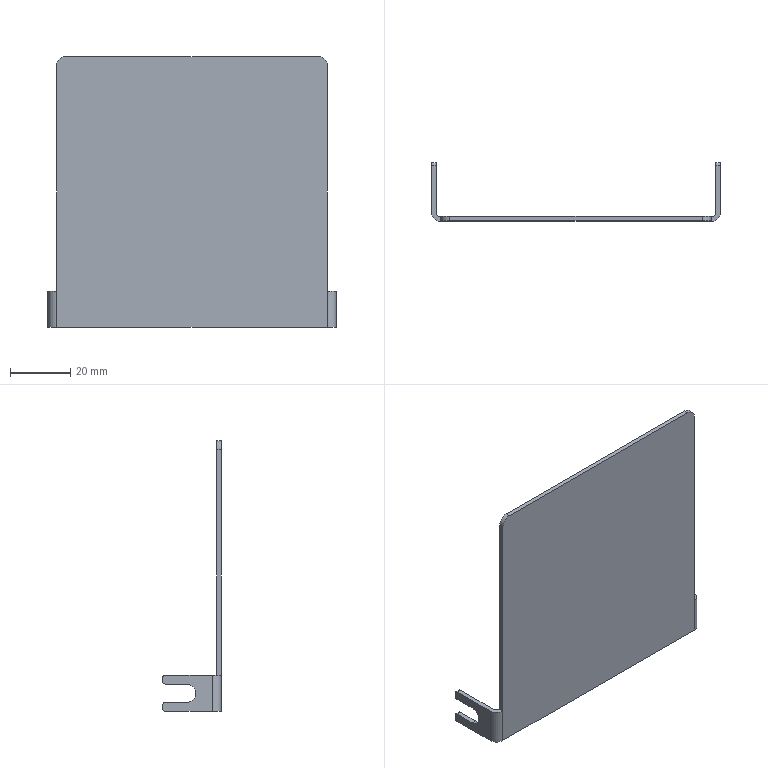Part | NX | features BREP 1 | 1 solid | 36 faces | box 96 x 19.5 x 90 mm | volume 12676 mm3 | plane 20 | cylinder 16 | commonest cylinder face diameters 2 x8 6 x6 3 x2
STEP:
#1=CARTESIAN_POINT('',(45.,0.,0.));
#2=VERTEX_POINT('',#1);
#3=CARTESIAN_POINT('',(-45.,0.,0.));
#4=VERTEX_POINT('',#3);
#5=CARTESIAN_POINT('',(-46.5,0.,0.));
#6=DIRECTION('',(-1.,0.,0.));
#7=VECTOR('',#6,1000.);
#8=LINE('',#5,#7);
#9=EDGE_CURVE('',#2,#4,#8,.T.);
#10=ORIENTED_EDGE('',*,*,#9,.T.);
#11=CARTESIAN_POINT('',(-45.,0.,12.));
#12=VERTEX_POINT('',#11);
#13=CARTESIAN_POINT('',(-45.,0.,90.));
#14=DIRECTION('',(0.,0.,1.));
#15=VECTOR('',#14,1000.);
#16=LINE('',#13,#15);
#17=EDGE_CURVE('',#4,#12,#16,.T.);
#18=ORIENTED_EDGE('',*,*,#17,.T.);
#19=CARTESIAN_POINT('',(-45.,0.,87.));
#20=VERTEX_POINT('',#19);
#21=CARTESIAN_POINT('',(-45.,0.,90.));
#22=DIRECTION('',(0.,0.,1.));
#23=VECTOR('',#22,1000.);
#24=LINE('',#21,#23);
#25=EDGE_CURVE('',#12,#20,#24,.T.);
#26=ORIENTED_EDGE('',*,*,#25,.T.);
#27=CARTESIAN_POINT('',(-42.,0.,90.));
#28=VERTEX_POINT('',#27);
#29=CARTESIAN_POINT('',(-42.,0.,87.));
#30=DIRECTION('',(0.,1.,0.));
#31=DIRECTION('',(1.,0.,0.));
#32=AXIS2_PLACEMENT_3D('',#29,#30,#31);
#33=CIRCLE('',#32,3.);
#34=EDGE_CURVE('',#20,#28,#33,.T.);
#35=ORIENTED_EDGE('',*,*,#34,.T.);
#36=CARTESIAN_POINT('',(42.,0.,90.));
#37=VERTEX_POINT('',#36);
#38=CARTESIAN_POINT('',(-46.5,0.,90.));
#39=DIRECTION('',(1.,0.,0.));
#40=VECTOR('',#39,1000.);
#41=LINE('',#38,#40);
#42=EDGE_CURVE('',#28,#37,#41,.T.);
#43=ORIENTED_EDGE('',*,*,#42,.T.);
#44=CARTESIAN_POINT('',(45.,0.,87.));
#45=VERTEX_POINT('',#44);
#46=CARTESIAN_POINT('',(42.,0.,87.));
#47=DIRECTION('',(0.,1.,0.));
#48=DIRECTION('',(-1.,0.,0.));
#49=AXIS2_PLACEMENT_3D('',#46,#47,#48);
#50=CIRCLE('',#49,3.);
#51=EDGE_CURVE('',#37,#45,#50,.T.);
#52=ORIENTED_EDGE('',*,*,#51,.T.);
#53=CARTESIAN_POINT('',(45.,0.,12.));
#54=VERTEX_POINT('',#53);
#55=CARTESIAN_POINT('',(45.,0.,90.));
#56=DIRECTION('',(0.,0.,-1.));
#57=VECTOR('',#56,1000.);
#58=LINE('',#55,#57);
#59=EDGE_CURVE('',#45,#54,#58,.T.);
#60=ORIENTED_EDGE('',*,*,#59,.T.);
#61=CARTESIAN_POINT('',(45.,0.,90.));
#62=DIRECTION('',(0.,0.,-1.));
#63=VECTOR('',#62,1000.);
#64=LINE('',#61,#63);
#65=EDGE_CURVE('',#54,#2,#64,.T.);
#66=ORIENTED_EDGE('',*,*,#65,.T.);
#67=EDGE_LOOP('',(#10,#18,#26,#35,#43,#52,#60,#66));
#68=FACE_BOUND('',#67,.T.);
#69=CARTESIAN_POINT('',(-46.5,0.,90.));
#70=DIRECTION('',(0.,1.,0.));
#71=DIRECTION('',(1.,0.,0.));
#72=AXIS2_PLACEMENT_3D('',#69,#70,#71);
#73=PLANE('',#72);
#74=ADVANCED_FACE('',(#68),#73,.T.);
#75=CARTESIAN_POINT('',(-46.5,1.5,12.));
#76=VERTEX_POINT('',#75);
#77=CARTESIAN_POINT('',(-45.,1.5,12.));
#78=DIRECTION('',(0.,0.,-1.));
#79=DIRECTION('',(-1.,0.,0.));
#80=AXIS2_PLACEMENT_3D('',#77,#78,#79);
#81=CIRCLE('',#80,1.5);
#82=EDGE_CURVE('',#12,#76,#81,.T.);
#83=ORIENTED_EDGE('',*,*,#82,.F.);
#84=ORIENTED_EDGE('',*,*,#17,.F.);
#85=CARTESIAN_POINT('',(-46.5,1.5,0.));
#86=VERTEX_POINT('',#85);
#87=CARTESIAN_POINT('',(-45.,1.5,0.));
#88=DIRECTION('',(0.,0.,1.));
#89=DIRECTION('',(-1.,0.,0.));
#90=AXIS2_PLACEMENT_3D('',#87,#88,#89);
#91=CIRCLE('',#90,1.5);
#92=EDGE_CURVE('',#86,#4,#91,.T.);
#93=ORIENTED_EDGE('',*,*,#92,.F.);
#94=CARTESIAN_POINT('',(-46.5,1.5,90.));
#95=DIRECTION('',(0.,0.,-1.));
#96=VECTOR('',#95,1000.);
#97=LINE('',#94,#96);
#98=EDGE_CURVE('',#76,#86,#97,.T.);
#99=ORIENTED_EDGE('',*,*,#98,.F.);
#100=EDGE_LOOP('',(#83,#84,#93,#99));
#101=FACE_BOUND('',#100,.T.);
#102=CARTESIAN_POINT('',(-45.,1.5,90.));
#103=DIRECTION('',(0.,0.,-1.));
#104=DIRECTION('',(1.,0.,0.));
#105=AXIS2_PLACEMENT_3D('',#102,#103,#104);
#106=CYLINDRICAL_SURFACE('',#105,1.5);
#107=ADVANCED_FACE('',(#101),#106,.F.);
#108=CARTESIAN_POINT('',(45.,-1.5,0.));
#109=VERTEX_POINT('',#108);
#110=CARTESIAN_POINT('',(-45.,-1.5,0.));
#111=VERTEX_POINT('',#110);
#112=CARTESIAN_POINT('',(48.,-1.5,0.));
#113=DIRECTION('',(-1.,0.,0.));
#114=VECTOR('',#113,1000.);
#115=LINE('',#112,#114);
#116=EDGE_CURVE('',#109,#111,#115,.T.);
#117=ORIENTED_EDGE('',*,*,#116,.T.);
#118=CARTESIAN_POINT('',(-48.,1.5,0.));
#119=VERTEX_POINT('',#118);
#120=CARTESIAN_POINT('',(-45.,1.5,0.));
#121=DIRECTION('',(0.,0.,-1.));
#122=DIRECTION('',(-1.,0.,0.));
#123=AXIS2_PLACEMENT_3D('',#120,#121,#122);
#124=CIRCLE('',#123,3.);
#125=EDGE_CURVE('',#111,#119,#124,.T.);
#126=ORIENTED_EDGE('',*,*,#125,.T.);
#127=CARTESIAN_POINT('',(-48.,17.,0.));
#128=VERTEX_POINT('',#127);
#129=CARTESIAN_POINT('',(-48.,-1.5,0.));
#130=DIRECTION('',(0.,1.,0.));
#131=VECTOR('',#130,1000.);
#132=LINE('',#129,#131);
#133=EDGE_CURVE('',#119,#128,#132,.T.);
#134=ORIENTED_EDGE('',*,*,#133,.T.);
#135=CARTESIAN_POINT('',(-46.5,17.,0.));
#136=VERTEX_POINT('',#135);
#137=CARTESIAN_POINT('',(-45.,17.,0.));
#138=DIRECTION('',(-1.,0.,0.));
#139=VECTOR('',#138,1000.);
#140=LINE('',#137,#139);
#141=EDGE_CURVE('',#136,#128,#140,.T.);
#142=ORIENTED_EDGE('',*,*,#141,.F.);
#143=CARTESIAN_POINT('',(-46.5,18.,0.));
#144=DIRECTION('',(0.,1.,0.));
#145=VECTOR('',#144,1000.);
#146=LINE('',#143,#145);
#147=EDGE_CURVE('',#86,#136,#146,.T.);
#148=ORIENTED_EDGE('',*,*,#147,.F.);
#149=ORIENTED_EDGE('',*,*,#92,.T.);
#150=ORIENTED_EDGE('',*,*,#9,.F.);
#151=CARTESIAN_POINT('',(46.5,1.5,0.));
#152=VERTEX_POINT('',#151);
#153=CARTESIAN_POINT('',(45.,1.5,0.));
#154=DIRECTION('',(0.,0.,1.));
#155=DIRECTION('',(-1.,0.,0.));
#156=AXIS2_PLACEMENT_3D('',#153,#154,#155);
#157=CIRCLE('',#156,1.5);
#158=EDGE_CURVE('',#2,#152,#157,.T.);
#159=ORIENTED_EDGE('',*,*,#158,.T.);
#160=CARTESIAN_POINT('',(46.5,17.,0.));
#161=VERTEX_POINT('',#160);
#162=CARTESIAN_POINT('',(46.5,0.,0.));
#163=DIRECTION('',(0.,-1.,0.));
#164=VECTOR('',#163,1000.);
#165=LINE('',#162,#164);
#166=EDGE_CURVE('',#161,#152,#165,.T.);
#167=ORIENTED_EDGE('',*,*,#166,.F.);
#168=CARTESIAN_POINT('',(48.,17.,0.));
#169=VERTEX_POINT('',#168);
#170=CARTESIAN_POINT('',(45.,17.,0.));
#171=DIRECTION('',(1.,0.,0.));
#172=VECTOR('',#171,1000.);
#173=LINE('',#170,#172);
#174=EDGE_CURVE('',#161,#169,#173,.T.);
#175=ORIENTED_EDGE('',*,*,#174,.T.);
#176=CARTESIAN_POINT('',(48.,1.5,0.));
#177=VERTEX_POINT('',#176);
#178=CARTESIAN_POINT('',(48.,0.,0.));
#179=DIRECTION('',(0.,-1.,0.));
#180=VECTOR('',#179,1000.);
#181=LINE('',#178,#180);
#182=EDGE_CURVE('',#169,#177,#181,.T.);
#183=ORIENTED_EDGE('',*,*,#182,.T.);
#184=CARTESIAN_POINT('',(45.,1.5,0.));
#185=DIRECTION('',(0.,0.,-1.));
#186=DIRECTION('',(-1.,0.,0.));
#187=AXIS2_PLACEMENT_3D('',#184,#185,#186);
#188=CIRCLE('',#187,3.);
#189=EDGE_CURVE('',#177,#109,#188,.T.);
#190=ORIENTED_EDGE('',*,*,#189,.T.);
#191=EDGE_LOOP('',(#117,#126,#134,#142,#148,#149,#150,#159,#167,#175,#183,#190));
#192=FACE_BOUND('',#191,.T.);
#193=CARTESIAN_POINT('',(48.,1.5,0.));
#194=DIRECTION('',(0.,0.,-1.));
#195=DIRECTION('',(1.,0.,0.));
#196=AXIS2_PLACEMENT_3D('',#193,#194,#195);
#197=PLANE('',#196);
#198=ADVANCED_FACE('',(#192),#197,.T.);
#199=CARTESIAN_POINT('',(46.5,1.5,12.));
#200=VERTEX_POINT('',#199);
#201=CARTESIAN_POINT('',(46.5,1.5,90.));
#202=DIRECTION('',(0.,0.,1.));
#203=VECTOR('',#202,1000.);
#204=LINE('',#201,#203);
#205=EDGE_CURVE('',#152,#200,#204,.T.);
#206=ORIENTED_EDGE('',*,*,#205,.F.);
#207=ORIENTED_EDGE('',*,*,#158,.F.);
#208=ORIENTED_EDGE('',*,*,#65,.F.);
#209=CARTESIAN_POINT('',(45.,1.5,12.));
#210=DIRECTION('',(0.,0.,-1.));
#211=DIRECTION('',(-1.,0.,0.));
#212=AXIS2_PLACEMENT_3D('',#209,#210,#211);
#213=CIRCLE('',#212,1.5);
#214=EDGE_CURVE('',#200,#54,#213,.T.);
#215=ORIENTED_EDGE('',*,*,#214,.F.);
#216=EDGE_LOOP('',(#206,#207,#208,#215));
#217=FACE_BOUND('',#216,.T.);
#218=CARTESIAN_POINT('',(45.,1.5,90.));
#219=DIRECTION('',(0.,0.,-1.));
#220=DIRECTION('',(1.,0.,0.));
#221=AXIS2_PLACEMENT_3D('',#218,#219,#220);
#222=CYLINDRICAL_SURFACE('',#221,1.5);
#223=ADVANCED_FACE('',(#217),#222,.F.);
#224=CARTESIAN_POINT('',(45.,-1.5,87.));
#225=VERTEX_POINT('',#224);
#226=CARTESIAN_POINT('',(45.,-1.5,12.));
#227=VERTEX_POINT('',#226);
#228=CARTESIAN_POINT('',(45.,-1.5,0.));
#229=DIRECTION('',(0.,0.,-1.));
#230=VECTOR('',#229,1000.);
#231=LINE('',#228,#230);
#232=EDGE_CURVE('',#225,#227,#231,.T.);
#233=ORIENTED_EDGE('',*,*,#232,.T.);
#234=CARTESIAN_POINT('',(45.,0.,12.));
#235=DIRECTION('',(0.,1.,0.));
#236=VECTOR('',#235,1000.);
#237=LINE('',#234,#236);
#238=EDGE_CURVE('',#227,#54,#237,.T.);
#239=ORIENTED_EDGE('',*,*,#238,.T.);
#240=ORIENTED_EDGE('',*,*,#59,.F.);
#241=CARTESIAN_POINT('',(45.,0.,87.));
#242=DIRECTION('',(0.,-1.,0.));
#243=VECTOR('',#242,1000.);
#244=LINE('',#241,#243);
#245=EDGE_CURVE('',#45,#225,#244,.T.);
#246=ORIENTED_EDGE('',*,*,#245,.T.);
#247=EDGE_LOOP('',(#233,#239,#240,#246));
#248=FACE_BOUND('',#247,.T.);
#249=CARTESIAN_POINT('',(45.,0.,0.));
#250=DIRECTION('',(1.,0.,0.));
#251=DIRECTION('',(0.,-1.,0.));
#252=AXIS2_PLACEMENT_3D('',#249,#250,#251);
#253=PLANE('',#252);
#254=ADVANCED_FACE('',(#248),#253,.T.);
#255=ORIENTED_EDGE('',*,*,#51,.F.);
#256=CARTESIAN_POINT('',(42.,-1.5,90.));
#257=VERTEX_POINT('',#256);
#258=CARTESIAN_POINT('',(42.,1.5,90.));
#259=DIRECTION('',(0.,-1.,0.));
#260=VECTOR('',#259,1000.);
#261=LINE('',#258,#260);
#262=EDGE_CURVE('',#37,#257,#261,.T.);
#263=ORIENTED_EDGE('',*,*,#262,.T.);
#264=CARTESIAN_POINT('',(42.,-1.5,87.));
#265=DIRECTION('',(0.,1.,0.));
#266=DIRECTION('',(-1.,0.,0.));
#267=AXIS2_PLACEMENT_3D('',#264,#265,#266);
#268=CIRCLE('',#267,3.);
#269=EDGE_CURVE('',#257,#225,#268,.T.);
#270=ORIENTED_EDGE('',*,*,#269,.T.);
#271=ORIENTED_EDGE('',*,*,#245,.F.);
#272=EDGE_LOOP('',(#255,#263,#270,#271));
#273=FACE_BOUND('',#272,.T.);
#274=CARTESIAN_POINT('',(42.,1.5,87.));
#275=DIRECTION('',(0.,1.,0.));
#276=DIRECTION('',(1.,0.,0.));
#277=AXIS2_PLACEMENT_3D('',#274,#275,#276);
#278=CYLINDRICAL_SURFACE('',#277,3.);
#279=ADVANCED_FACE('',(#273),#278,.T.);
#280=CARTESIAN_POINT('',(-42.,-1.5,90.));
#281=VERTEX_POINT('',#280);
#282=CARTESIAN_POINT('',(-48.,-1.5,90.));
#283=DIRECTION('',(1.,0.,0.));
#284=VECTOR('',#283,1000.);
#285=LINE('',#282,#284);
#286=EDGE_CURVE('',#281,#257,#285,.T.);
#287=ORIENTED_EDGE('',*,*,#286,.T.);
#288=ORIENTED_EDGE('',*,*,#262,.F.);
#289=ORIENTED_EDGE('',*,*,#42,.F.);
#290=CARTESIAN_POINT('',(-42.,1.5,90.));
#291=DIRECTION('',(0.,-1.,0.));
#292=VECTOR('',#291,1000.);
#293=LINE('',#290,#292);
#294=EDGE_CURVE('',#28,#281,#293,.T.);
#295=ORIENTED_EDGE('',*,*,#294,.T.);
#296=EDGE_LOOP('',(#287,#288,#289,#295));
#297=FACE_BOUND('',#296,.T.);
#298=CARTESIAN_POINT('',(-48.,1.5,90.));
#299=DIRECTION('',(0.,0.,1.));
#300=DIRECTION('',(-1.,0.,0.));
#301=AXIS2_PLACEMENT_3D('',#298,#299,#300);
#302=PLANE('',#301);
#303=ADVANCED_FACE('',(#297),#302,.T.);
#304=CARTESIAN_POINT('',(-45.,-1.5,87.));
#305=VERTEX_POINT('',#304);
#306=CARTESIAN_POINT('',(-42.,-1.5,87.));
#307=DIRECTION('',(0.,1.,0.));
#308=DIRECTION('',(1.,0.,0.));
#309=AXIS2_PLACEMENT_3D('',#306,#307,#308);
#310=CIRCLE('',#309,3.);
#311=EDGE_CURVE('',#305,#281,#310,.T.);
#312=ORIENTED_EDGE('',*,*,#311,.T.);
#313=ORIENTED_EDGE('',*,*,#294,.F.);
#314=ORIENTED_EDGE('',*,*,#34,.F.);
#315=CARTESIAN_POINT('',(-45.,1.5,87.));
#316=DIRECTION('',(0.,-1.,0.));
#317=VECTOR('',#316,1000.);
#318=LINE('',#315,#317);
#319=EDGE_CURVE('',#20,#305,#318,.T.);
#320=ORIENTED_EDGE('',*,*,#319,.T.);
#321=EDGE_LOOP('',(#312,#313,#314,#320));
#322=FACE_BOUND('',#321,.T.);
#323=CARTESIAN_POINT('',(-42.,1.5,87.));
#324=DIRECTION('',(0.,-1.,0.));
#325=DIRECTION('',(-1.,0.,0.));
#326=AXIS2_PLACEMENT_3D('',#323,#324,#325);
#327=CYLINDRICAL_SURFACE('',#326,3.);
#328=ADVANCED_FACE('',(#322),#327,.T.);
#329=ORIENTED_EDGE('',*,*,#25,.F.);
#330=CARTESIAN_POINT('',(-45.,-1.5,12.));
#331=VERTEX_POINT('',#330);
#332=CARTESIAN_POINT('',(-45.,0.,12.));
#333=DIRECTION('',(0.,-1.,0.));
#334=VECTOR('',#333,1000.);
#335=LINE('',#332,#334);
#336=EDGE_CURVE('',#12,#331,#335,.T.);
#337=ORIENTED_EDGE('',*,*,#336,.T.);
#338=CARTESIAN_POINT('',(-45.,-1.5,0.));
#339=DIRECTION('',(0.,0.,1.));
#340=VECTOR('',#339,1000.);
#341=LINE('',#338,#340);
#342=EDGE_CURVE('',#331,#305,#341,.T.);
#343=ORIENTED_EDGE('',*,*,#342,.T.);
#344=ORIENTED_EDGE('',*,*,#319,.F.);
#345=EDGE_LOOP('',(#329,#337,#343,#344));
#346=FACE_BOUND('',#345,.T.);
#347=CARTESIAN_POINT('',(-45.,0.,0.));
#348=DIRECTION('',(-1.,0.,0.));
#349=DIRECTION('',(0.,1.,0.));
#350=AXIS2_PLACEMENT_3D('',#347,#348,#349);
#351=PLANE('',#350);
#352=ADVANCED_FACE('',(#346),#351,.T.);
#353=CARTESIAN_POINT('',(-46.5,17.,12.));
#354=VERTEX_POINT('',#353);
#355=CARTESIAN_POINT('',(-46.5,18.,12.));
#356=DIRECTION('',(0.,-1.,0.));
#357=VECTOR('',#356,1000.);
#358=LINE('',#355,#357);
#359=EDGE_CURVE('',#354,#76,#358,.T.);
#360=ORIENTED_EDGE('',*,*,#359,.T.);
#361=ORIENTED_EDGE('',*,*,#98,.T.);
#362=ORIENTED_EDGE('',*,*,#147,.T.);
#363=CARTESIAN_POINT('',(-46.5,18.,1.));
#364=VERTEX_POINT('',#363);
#365=CARTESIAN_POINT('',(-46.5,17.,1.));
#366=DIRECTION('',(1.,0.,0.));
#367=DIRECTION('',(0.,0.,-1.));
#368=AXIS2_PLACEMENT_3D('',#365,#366,#367);
#369=CIRCLE('',#368,1.);
#370=EDGE_CURVE('',#136,#364,#369,.T.);
#371=ORIENTED_EDGE('',*,*,#370,.T.);
#372=CARTESIAN_POINT('',(-46.5,18.,2.));
#373=VERTEX_POINT('',#372);
#374=CARTESIAN_POINT('',(-46.5,18.,90.));
#375=DIRECTION('',(0.,0.,1.));
#376=VECTOR('',#375,1000.);
#377=LINE('',#374,#376);
#378=EDGE_CURVE('',#364,#373,#377,.T.);
#379=ORIENTED_EDGE('',*,*,#378,.T.);
#380=CARTESIAN_POINT('',(-46.5,17.,3.));
#381=VERTEX_POINT('',#380);
#382=CARTESIAN_POINT('',(-46.5,17.,2.));
#383=DIRECTION('',(1.,0.,0.));
#384=DIRECTION('',(0.,0.,1.));
#385=AXIS2_PLACEMENT_3D('',#382,#383,#384);
#386=CIRCLE('',#385,1.);
#387=EDGE_CURVE('',#373,#381,#386,.T.);
#388=ORIENTED_EDGE('',*,*,#387,.T.);
#389=CARTESIAN_POINT('',(-46.5,10.,3.));
#390=VERTEX_POINT('',#389);
#391=CARTESIAN_POINT('',(-46.5,18.,3.));
#392=DIRECTION('',(0.,-1.,0.));
#393=VECTOR('',#392,1000.);
#394=LINE('',#391,#393);
#395=EDGE_CURVE('',#381,#390,#394,.T.);
#396=ORIENTED_EDGE('',*,*,#395,.T.);
#397=CARTESIAN_POINT('',(-46.5,10.,9.));
#398=VERTEX_POINT('',#397);
#399=CARTESIAN_POINT('',(-46.5,10.,6.));
#400=DIRECTION('',(-1.,0.,0.));
#401=DIRECTION('',(0.,1.,0.));
#402=AXIS2_PLACEMENT_3D('',#399,#400,#401);
#403=CIRCLE('',#402,3.);
#404=EDGE_CURVE('',#390,#398,#403,.T.);
#405=ORIENTED_EDGE('',*,*,#404,.T.);
#406=CARTESIAN_POINT('',(-46.5,17.,9.));
#407=VERTEX_POINT('',#406);
#408=CARTESIAN_POINT('',(-46.5,18.,9.));
#409=DIRECTION('',(0.,1.,0.));
#410=VECTOR('',#409,1000.);
#411=LINE('',#408,#410);
#412=EDGE_CURVE('',#398,#407,#411,.T.);
#413=ORIENTED_EDGE('',*,*,#412,.T.);
#414=CARTESIAN_POINT('',(-46.5,18.,10.));
#415=VERTEX_POINT('',#414);
#416=CARTESIAN_POINT('',(-46.5,17.,10.));
#417=DIRECTION('',(1.,0.,0.));
#418=DIRECTION('',(0.,0.,1.));
#419=AXIS2_PLACEMENT_3D('',#416,#417,#418);
#420=CIRCLE('',#419,1.);
#421=EDGE_CURVE('',#407,#415,#420,.T.);
#422=ORIENTED_EDGE('',*,*,#421,.T.);
#423=CARTESIAN_POINT('',(-46.5,18.,11.));
#424=VERTEX_POINT('',#423);
#425=CARTESIAN_POINT('',(-46.5,18.,90.));
#426=DIRECTION('',(0.,0.,1.));
#427=VECTOR('',#426,1000.);
#428=LINE('',#425,#427);
#429=EDGE_CURVE('',#415,#424,#428,.T.);
#430=ORIENTED_EDGE('',*,*,#429,.T.);
#431=CARTESIAN_POINT('',(-46.5,17.,11.));
#432=DIRECTION('',(1.,0.,0.));
#433=DIRECTION('',(0.,0.,1.));
#434=AXIS2_PLACEMENT_3D('',#431,#432,#433);
#435=CIRCLE('',#434,1.);
#436=EDGE_CURVE('',#424,#354,#435,.T.);
#437=ORIENTED_EDGE('',*,*,#436,.T.);
#438=EDGE_LOOP('',(#360,#361,#362,#371,#379,#388,#396,#405,#413,#422,#430,#437));
#439=FACE_BOUND('',#438,.T.);
#440=CARTESIAN_POINT('',(-46.5,18.,90.));
#441=DIRECTION('',(1.,0.,0.));
#442=DIRECTION('',(0.,-1.,0.));
#443=AXIS2_PLACEMENT_3D('',#440,#441,#442);
#444=PLANE('',#443);
#445=ADVANCED_FACE('',(#439),#444,.T.);
#446=ORIENTED_EDGE('',*,*,#336,.F.);
#447=ORIENTED_EDGE('',*,*,#82,.T.);
#448=ORIENTED_EDGE('',*,*,#359,.F.);
#449=CARTESIAN_POINT('',(-48.,17.,12.));
#450=VERTEX_POINT('',#449);
#451=CARTESIAN_POINT('',(-45.,17.,12.));
#452=DIRECTION('',(-1.,0.,0.));
#453=VECTOR('',#452,1000.);
#454=LINE('',#451,#453);
#455=EDGE_CURVE('',#354,#450,#454,.T.);
#456=ORIENTED_EDGE('',*,*,#455,.T.);
#457=CARTESIAN_POINT('',(-48.,1.5,12.));
#458=VERTEX_POINT('',#457);
#459=CARTESIAN_POINT('',(-48.,-1.5,12.));
#460=DIRECTION('',(0.,-1.,0.));
#461=VECTOR('',#460,1000.);
#462=LINE('',#459,#461);
#463=EDGE_CURVE('',#450,#458,#462,.T.);
#464=ORIENTED_EDGE('',*,*,#463,.T.);
#465=CARTESIAN_POINT('',(-45.,1.5,12.));
#466=DIRECTION('',(0.,0.,1.));
#467=DIRECTION('',(-1.,0.,0.));
#468=AXIS2_PLACEMENT_3D('',#465,#466,#467);
#469=CIRCLE('',#468,3.);
#470=EDGE_CURVE('',#458,#331,#469,.T.);
#471=ORIENTED_EDGE('',*,*,#470,.T.);
#472=EDGE_LOOP('',(#446,#447,#448,#456,#464,#471));
#473=FACE_BOUND('',#472,.T.);
#474=CARTESIAN_POINT('',(-45.,-1.5,12.));
#475=DIRECTION('',(0.,0.,1.));
#476=DIRECTION('',(-1.,0.,0.));
#477=AXIS2_PLACEMENT_3D('',#474,#475,#476);
#478=PLANE('',#477);
#479=ADVANCED_FACE('',(#473),#478,.T.);
#480=ORIENTED_EDGE('',*,*,#311,.F.);
#481=ORIENTED_EDGE('',*,*,#342,.F.);
#482=CARTESIAN_POINT('',(-45.,-1.5,90.));
#483=DIRECTION('',(0.,0.,1.));
#484=VECTOR('',#483,1000.);
#485=LINE('',#482,#484);
#486=EDGE_CURVE('',#111,#331,#485,.T.);
#487=ORIENTED_EDGE('',*,*,#486,.F.);
#488=ORIENTED_EDGE('',*,*,#116,.F.);
#489=CARTESIAN_POINT('',(45.,-1.5,90.));
#490=DIRECTION('',(0.,0.,-1.));
#491=VECTOR('',#490,1000.);
#492=LINE('',#489,#491);
#493=EDGE_CURVE('',#227,#109,#492,.T.);
#494=ORIENTED_EDGE('',*,*,#493,.F.);
#495=ORIENTED_EDGE('',*,*,#232,.F.);
#496=ORIENTED_EDGE('',*,*,#269,.F.);
#497=ORIENTED_EDGE('',*,*,#286,.F.);
#498=EDGE_LOOP('',(#480,#481,#487,#488,#494,#495,#496,#497));
#499=FACE_BOUND('',#498,.T.);
#500=CARTESIAN_POINT('',(-46.5,-1.5,90.));
#501=DIRECTION('',(0.,1.,0.));
#502=DIRECTION('',(1.,0.,0.));
#503=AXIS2_PLACEMENT_3D('',#500,#501,#502);
#504=PLANE('',#503);
#505=ADVANCED_FACE('',(#499),#504,.F.);
#506=CARTESIAN_POINT('',(46.5,17.,12.));
#507=VERTEX_POINT('',#506);
#508=CARTESIAN_POINT('',(48.,17.,12.));
#509=VERTEX_POINT('',#508);
#510=CARTESIAN_POINT('',(45.,17.,12.));
#511=DIRECTION('',(1.,0.,0.));
#512=VECTOR('',#511,1000.);
#513=LINE('',#510,#512);
#514=EDGE_CURVE('',#507,#509,#513,.T.);
#515=ORIENTED_EDGE('',*,*,#514,.F.);
#516=CARTESIAN_POINT('',(46.5,-1.5,12.));
#517=DIRECTION('',(0.,1.,0.));
#518=VECTOR('',#517,1000.);
#519=LINE('',#516,#518);
#520=EDGE_CURVE('',#200,#507,#519,.T.);
#521=ORIENTED_EDGE('',*,*,#520,.F.);
#522=ORIENTED_EDGE('',*,*,#214,.T.);
#523=ORIENTED_EDGE('',*,*,#238,.F.);
#524=CARTESIAN_POINT('',(48.,1.5,12.));
#525=VERTEX_POINT('',#524);
#526=CARTESIAN_POINT('',(45.,1.5,12.));
#527=DIRECTION('',(0.,0.,-1.));
#528=DIRECTION('',(-1.,0.,0.));
#529=AXIS2_PLACEMENT_3D('',#526,#527,#528);
#530=CIRCLE('',#529,3.);
#531=EDGE_CURVE('',#525,#227,#530,.T.);
#532=ORIENTED_EDGE('',*,*,#531,.F.);
#533=CARTESIAN_POINT('',(48.,-1.5,12.));
#534=DIRECTION('',(0.,-1.,0.));
#535=VECTOR('',#534,1000.);
#536=LINE('',#533,#535);
#537=EDGE_CURVE('',#509,#525,#536,.T.);
#538=ORIENTED_EDGE('',*,*,#537,.F.);
#539=EDGE_LOOP('',(#515,#521,#522,#523,#532,#538));
#540=FACE_BOUND('',#539,.T.);
#541=CARTESIAN_POINT('',(45.,-1.5,12.));
#542=DIRECTION('',(0.,0.,-1.));
#543=DIRECTION('',(1.,0.,0.));
#544=AXIS2_PLACEMENT_3D('',#541,#542,#543);
#545=PLANE('',#544);
#546=ADVANCED_FACE('',(#540),#545,.F.);
#547=ORIENTED_EDGE('',*,*,#166,.T.);
#548=ORIENTED_EDGE('',*,*,#205,.T.);
#549=ORIENTED_EDGE('',*,*,#520,.T.);
#550=CARTESIAN_POINT('',(46.5,18.,11.));
#551=VERTEX_POINT('',#550);
#552=CARTESIAN_POINT('',(46.5,17.,11.));
#553=DIRECTION('',(-1.,0.,0.));
#554=DIRECTION('',(0.,0.,1.));
#555=AXIS2_PLACEMENT_3D('',#552,#553,#554);
#556=CIRCLE('',#555,1.);
#557=EDGE_CURVE('',#507,#551,#556,.T.);
#558=ORIENTED_EDGE('',*,*,#557,.T.);
#559=CARTESIAN_POINT('',(46.5,18.,10.));
#560=VERTEX_POINT('',#559);
#561=CARTESIAN_POINT('',(46.5,18.,90.));
#562=DIRECTION('',(0.,0.,-1.));
#563=VECTOR('',#562,1000.);
#564=LINE('',#561,#563);
#565=EDGE_CURVE('',#551,#560,#564,.T.);
#566=ORIENTED_EDGE('',*,*,#565,.T.);
#567=CARTESIAN_POINT('',(46.5,17.,9.));
#568=VERTEX_POINT('',#567);
#569=CARTESIAN_POINT('',(46.5,17.,10.));
#570=DIRECTION('',(-1.,0.,0.));
#571=DIRECTION('',(0.,0.,1.));
#572=AXIS2_PLACEMENT_3D('',#569,#570,#571);
#573=CIRCLE('',#572,1.);
#574=EDGE_CURVE('',#560,#568,#573,.T.);
#575=ORIENTED_EDGE('',*,*,#574,.T.);
#576=CARTESIAN_POINT('',(46.5,10.,9.));
#577=VERTEX_POINT('',#576);
#578=CARTESIAN_POINT('',(46.5,0.,9.));
#579=DIRECTION('',(0.,-1.,0.));
#580=VECTOR('',#579,1000.);
#581=LINE('',#578,#580);
#582=EDGE_CURVE('',#568,#577,#581,.T.);
#583=ORIENTED_EDGE('',*,*,#582,.T.);
#584=CARTESIAN_POINT('',(46.5,10.,3.));
#585=VERTEX_POINT('',#584);
#586=CARTESIAN_POINT('',(46.5,10.,6.));
#587=DIRECTION('',(1.,0.,0.));
#588=DIRECTION('',(0.,1.,0.));
#589=AXIS2_PLACEMENT_3D('',#586,#587,#588);
#590=CIRCLE('',#589,3.);
#591=EDGE_CURVE('',#577,#585,#590,.T.);
#592=ORIENTED_EDGE('',*,*,#591,.T.);
#593=CARTESIAN_POINT('',(46.5,17.,3.));
#594=VERTEX_POINT('',#593);
#595=CARTESIAN_POINT('',(46.5,0.,3.));
#596=DIRECTION('',(0.,1.,0.));
#597=VECTOR('',#596,1000.);
#598=LINE('',#595,#597);
#599=EDGE_CURVE('',#585,#594,#598,.T.);
#600=ORIENTED_EDGE('',*,*,#599,.T.);
#601=CARTESIAN_POINT('',(46.5,18.,2.));
#602=VERTEX_POINT('',#601);
#603=CARTESIAN_POINT('',(46.5,17.,2.));
#604=DIRECTION('',(-1.,0.,0.));
#605=DIRECTION('',(0.,0.,1.));
#606=AXIS2_PLACEMENT_3D('',#603,#604,#605);
#607=CIRCLE('',#606,1.);
#608=EDGE_CURVE('',#594,#602,#607,.T.);
#609=ORIENTED_EDGE('',*,*,#608,.T.);
#610=CARTESIAN_POINT('',(46.5,18.,1.));
#611=VERTEX_POINT('',#610);
#612=CARTESIAN_POINT('',(46.5,18.,90.));
#613=DIRECTION('',(0.,0.,-1.));
#614=VECTOR('',#613,1000.);
#615=LINE('',#612,#614);
#616=EDGE_CURVE('',#602,#611,#615,.T.);
#617=ORIENTED_EDGE('',*,*,#616,.T.);
#618=CARTESIAN_POINT('',(46.5,17.,1.));
#619=DIRECTION('',(-1.,0.,0.));
#620=DIRECTION('',(0.,0.,-1.));
#621=AXIS2_PLACEMENT_3D('',#618,#619,#620);
#622=CIRCLE('',#621,1.);
#623=EDGE_CURVE('',#611,#161,#622,.T.);
#624=ORIENTED_EDGE('',*,*,#623,.T.);
#625=EDGE_LOOP('',(#547,#548,#549,#558,#566,#575,#583,#592,#600,#609,#617,#624));
#626=FACE_BOUND('',#625,.T.);
#627=CARTESIAN_POINT('',(46.5,0.,90.));
#628=DIRECTION('',(-1.,0.,0.));
#629=DIRECTION('',(0.,1.,0.));
#630=AXIS2_PLACEMENT_3D('',#627,#628,#629);
#631=PLANE('',#630);
#632=ADVANCED_FACE('',(#626),#631,.T.);
#633=CARTESIAN_POINT('',(-48.,18.,11.));
#634=VERTEX_POINT('',#633);
#635=CARTESIAN_POINT('',(-48.,17.,11.));
#636=DIRECTION('',(1.,0.,0.));
#637=DIRECTION('',(0.,0.,1.));
#638=AXIS2_PLACEMENT_3D('',#635,#636,#637);
#639=CIRCLE('',#638,1.);
#640=EDGE_CURVE('',#634,#450,#639,.T.);
#641=ORIENTED_EDGE('',*,*,#640,.T.);
#642=ORIENTED_EDGE('',*,*,#455,.F.);
#643=ORIENTED_EDGE('',*,*,#436,.F.);
#644=CARTESIAN_POINT('',(-45.,18.,11.));
#645=DIRECTION('',(-1.,0.,0.));
#646=VECTOR('',#645,1000.);
#647=LINE('',#644,#646);
#648=EDGE_CURVE('',#424,#634,#647,.T.);
#649=ORIENTED_EDGE('',*,*,#648,.T.);
#650=EDGE_LOOP('',(#641,#642,#643,#649));
#651=FACE_BOUND('',#650,.T.);
#652=CARTESIAN_POINT('',(-45.,17.,11.));
#653=DIRECTION('',(-1.,0.,0.));
#654=DIRECTION('',(0.,0.,-1.));
#655=AXIS2_PLACEMENT_3D('',#652,#653,#654);
#656=CYLINDRICAL_SURFACE('',#655,1.);
#657=ADVANCED_FACE('',(#651),#656,.T.);
#658=ORIENTED_EDGE('',*,*,#429,.F.);
#659=CARTESIAN_POINT('',(-48.,18.,10.));
#660=VERTEX_POINT('',#659);
#661=CARTESIAN_POINT('',(-48.,18.,10.));
#662=DIRECTION('',(-1.,0.,0.));
#663=VECTOR('',#662,1000.);
#664=LINE('',#661,#663);
#665=EDGE_CURVE('',#415,#660,#664,.T.);
#666=ORIENTED_EDGE('',*,*,#665,.T.);
#667=CARTESIAN_POINT('',(-48.,18.,90.));
#668=DIRECTION('',(0.,0.,1.));
#669=VECTOR('',#668,1000.);
#670=LINE('',#667,#669);
#671=EDGE_CURVE('',#660,#634,#670,.T.);
#672=ORIENTED_EDGE('',*,*,#671,.T.);
#673=ORIENTED_EDGE('',*,*,#648,.F.);
#674=EDGE_LOOP('',(#658,#666,#672,#673));
#675=FACE_BOUND('',#674,.T.);
#676=CARTESIAN_POINT('',(-48.,18.,90.));
#677=DIRECTION('',(0.,1.,0.));
#678=DIRECTION('',(0.,0.,-1.));
#679=AXIS2_PLACEMENT_3D('',#676,#677,#678);
#680=PLANE('',#679);
#681=ADVANCED_FACE('',(#675),#680,.T.);
#682=ORIENTED_EDGE('',*,*,#421,.F.);
#683=CARTESIAN_POINT('',(-48.,17.,9.));
#684=VERTEX_POINT('',#683);
#685=CARTESIAN_POINT('',(-48.,17.,9.));
#686=DIRECTION('',(-1.,0.,0.));
#687=VECTOR('',#686,1000.);
#688=LINE('',#685,#687);
#689=EDGE_CURVE('',#407,#684,#688,.T.);
#690=ORIENTED_EDGE('',*,*,#689,.T.);
#691=CARTESIAN_POINT('',(-48.,17.,10.));
#692=DIRECTION('',(1.,0.,0.));
#693=DIRECTION('',(0.,0.,1.));
#694=AXIS2_PLACEMENT_3D('',#691,#692,#693);
#695=CIRCLE('',#694,1.);
#696=EDGE_CURVE('',#684,#660,#695,.T.);
#697=ORIENTED_EDGE('',*,*,#696,.T.);
#698=ORIENTED_EDGE('',*,*,#665,.F.);
#699=EDGE_LOOP('',(#682,#690,#697,#698));
#700=FACE_BOUND('',#699,.T.);
#701=CARTESIAN_POINT('',(-48.,17.,10.));
#702=DIRECTION('',(-1.,0.,0.));
#703=DIRECTION('',(0.,0.,-1.));
#704=AXIS2_PLACEMENT_3D('',#701,#702,#703);
#705=CYLINDRICAL_SURFACE('',#704,1.);
#706=ADVANCED_FACE('',(#700),#705,.T.);
#707=ORIENTED_EDGE('',*,*,#689,.F.);
#708=ORIENTED_EDGE('',*,*,#412,.F.);
#709=CARTESIAN_POINT('',(-48.,10.,9.));
#710=VERTEX_POINT('',#709);
#711=CARTESIAN_POINT('',(-48.,10.,9.));
#712=DIRECTION('',(1.,0.,0.));
#713=VECTOR('',#712,1000.);
#714=LINE('',#711,#713);
#715=EDGE_CURVE('',#710,#398,#714,.T.);
#716=ORIENTED_EDGE('',*,*,#715,.F.);
#717=CARTESIAN_POINT('',(-48.,18.,9.));
#718=DIRECTION('',(0.,-1.,0.));
#719=VECTOR('',#718,1000.);
#720=LINE('',#717,#719);
#721=EDGE_CURVE('',#684,#710,#720,.T.);
#722=ORIENTED_EDGE('',*,*,#721,.F.);
#723=EDGE_LOOP('',(#707,#708,#716,#722));
#724=FACE_BOUND('',#723,.T.);
#725=CARTESIAN_POINT('',(-48.,18.,9.));
#726=DIRECTION('',(0.,0.,1.));
#727=DIRECTION('',(-1.,0.,0.));
#728=AXIS2_PLACEMENT_3D('',#725,#726,#727);
#729=PLANE('',#728);
#730=ADVANCED_FACE('',(#724),#729,.F.);
#731=CARTESIAN_POINT('',(-48.,10.,3.));
#732=VERTEX_POINT('',#731);
#733=CARTESIAN_POINT('',(-48.,10.,3.));
#734=DIRECTION('',(1.,0.,0.));
#735=VECTOR('',#734,1000.);
#736=LINE('',#733,#735);
#737=EDGE_CURVE('',#732,#390,#736,.T.);
#738=ORIENTED_EDGE('',*,*,#737,.F.);
#739=CARTESIAN_POINT('',(-48.,10.,6.));
#740=DIRECTION('',(1.,0.,0.));
#741=DIRECTION('',(0.,1.,0.));
#742=AXIS2_PLACEMENT_3D('',#739,#740,#741);
#743=CIRCLE('',#742,3.);
#744=EDGE_CURVE('',#710,#732,#743,.T.);
#745=ORIENTED_EDGE('',*,*,#744,.F.);
#746=ORIENTED_EDGE('',*,*,#715,.T.);
#747=ORIENTED_EDGE('',*,*,#404,.F.);
#748=EDGE_LOOP('',(#738,#745,#746,#747));
#749=FACE_BOUND('',#748,.T.);
#750=CARTESIAN_POINT('',(-48.,10.,6.));
#751=DIRECTION('',(1.,0.,0.));
#752=DIRECTION('',(0.,-1.,0.));
#753=AXIS2_PLACEMENT_3D('',#750,#751,#752);
#754=CYLINDRICAL_SURFACE('',#753,3.);
#755=ADVANCED_FACE('',(#749),#754,.F.);
#756=CARTESIAN_POINT('',(-48.,17.,3.));
#757=VERTEX_POINT('',#756);
#758=CARTESIAN_POINT('',(-48.,17.,3.));
#759=DIRECTION('',(1.,0.,0.));
#760=VECTOR('',#759,1000.);
#761=LINE('',#758,#760);
#762=EDGE_CURVE('',#757,#381,#761,.T.);
#763=ORIENTED_EDGE('',*,*,#762,.F.);
#764=CARTESIAN_POINT('',(-48.,18.,3.));
#765=DIRECTION('',(0.,1.,0.));
#766=VECTOR('',#765,1000.);
#767=LINE('',#764,#766);
#768=EDGE_CURVE('',#732,#757,#767,.T.);
#769=ORIENTED_EDGE('',*,*,#768,.F.);
#770=ORIENTED_EDGE('',*,*,#737,.T.);
#771=ORIENTED_EDGE('',*,*,#395,.F.);
#772=EDGE_LOOP('',(#763,#769,#770,#771));
#773=FACE_BOUND('',#772,.T.);
#774=CARTESIAN_POINT('',(-48.,18.,3.));
#775=DIRECTION('',(0.,0.,-1.));
#776=DIRECTION('',(0.,-1.,0.));
#777=AXIS2_PLACEMENT_3D('',#774,#775,#776);
#778=PLANE('',#777);
#779=ADVANCED_FACE('',(#773),#778,.F.);
#780=ORIENTED_EDGE('',*,*,#387,.F.);
#781=CARTESIAN_POINT('',(-48.,18.,2.));
#782=VERTEX_POINT('',#781);
#783=CARTESIAN_POINT('',(-48.,18.,2.));
#784=DIRECTION('',(-1.,0.,0.));
#785=VECTOR('',#784,1000.);
#786=LINE('',#783,#785);
#787=EDGE_CURVE('',#373,#782,#786,.T.);
#788=ORIENTED_EDGE('',*,*,#787,.T.);
#789=CARTESIAN_POINT('',(-48.,17.,2.));
#790=DIRECTION('',(1.,0.,0.));
#791=DIRECTION('',(0.,0.,1.));
#792=AXIS2_PLACEMENT_3D('',#789,#790,#791);
#793=CIRCLE('',#792,1.);
#794=EDGE_CURVE('',#782,#757,#793,.T.);
#795=ORIENTED_EDGE('',*,*,#794,.T.);
#796=ORIENTED_EDGE('',*,*,#762,.T.);
#797=EDGE_LOOP('',(#780,#788,#795,#796));
#798=FACE_BOUND('',#797,.T.);
#799=CARTESIAN_POINT('',(-48.,17.,2.));
#800=DIRECTION('',(-1.,0.,0.));
#801=DIRECTION('',(0.,0.,-1.));
#802=AXIS2_PLACEMENT_3D('',#799,#800,#801);
#803=CYLINDRICAL_SURFACE('',#802,1.);
#804=ADVANCED_FACE('',(#798),#803,.T.);
#805=CARTESIAN_POINT('',(-48.,18.,1.));
#806=VERTEX_POINT('',#805);
#807=CARTESIAN_POINT('',(-48.,18.,90.));
#808=DIRECTION('',(0.,0.,1.));
#809=VECTOR('',#808,1000.);
#810=LINE('',#807,#809);
#811=EDGE_CURVE('',#806,#782,#810,.T.);
#812=ORIENTED_EDGE('',*,*,#811,.T.);
#813=ORIENTED_EDGE('',*,*,#787,.F.);
#814=ORIENTED_EDGE('',*,*,#378,.F.);
#815=CARTESIAN_POINT('',(-48.,18.,1.));
#816=DIRECTION('',(-1.,0.,0.));
#817=VECTOR('',#816,1000.);
#818=LINE('',#815,#817);
#819=EDGE_CURVE('',#364,#806,#818,.T.);
#820=ORIENTED_EDGE('',*,*,#819,.T.);
#821=EDGE_LOOP('',(#812,#813,#814,#820));
#822=FACE_BOUND('',#821,.T.);
#823=CARTESIAN_POINT('',(-48.,18.,90.));
#824=DIRECTION('',(0.,1.,0.));
#825=DIRECTION('',(0.,0.,-1.));
#826=AXIS2_PLACEMENT_3D('',#823,#824,#825);
#827=PLANE('',#826);
#828=ADVANCED_FACE('',(#822),#827,.T.);
#829=ORIENTED_EDGE('',*,*,#370,.F.);
#830=ORIENTED_EDGE('',*,*,#141,.T.);
#831=CARTESIAN_POINT('',(-48.,17.,1.));
#832=DIRECTION('',(1.,0.,0.));
#833=DIRECTION('',(0.,0.,-1.));
#834=AXIS2_PLACEMENT_3D('',#831,#832,#833);
#835=CIRCLE('',#834,1.);
#836=EDGE_CURVE('',#128,#806,#835,.T.);
#837=ORIENTED_EDGE('',*,*,#836,.T.);
#838=ORIENTED_EDGE('',*,*,#819,.F.);
#839=EDGE_LOOP('',(#829,#830,#837,#838));
#840=FACE_BOUND('',#839,.T.);
#841=CARTESIAN_POINT('',(-45.,17.,1.));
#842=DIRECTION('',(1.,0.,0.));
#843=DIRECTION('',(0.,0.,1.));
#844=AXIS2_PLACEMENT_3D('',#841,#842,#843);
#845=CYLINDRICAL_SURFACE('',#844,1.);
#846=ADVANCED_FACE('',(#840),#845,.T.);
#847=ORIENTED_EDGE('',*,*,#125,.F.);
#848=ORIENTED_EDGE('',*,*,#486,.T.);
#849=ORIENTED_EDGE('',*,*,#470,.F.);
#850=CARTESIAN_POINT('',(-48.,1.5,90.));
#851=DIRECTION('',(0.,0.,-1.));
#852=VECTOR('',#851,1000.);
#853=LINE('',#850,#852);
#854=EDGE_CURVE('',#458,#119,#853,.T.);
#855=ORIENTED_EDGE('',*,*,#854,.T.);
#856=EDGE_LOOP('',(#847,#848,#849,#855));
#857=FACE_BOUND('',#856,.T.);
#858=CARTESIAN_POINT('',(-45.,1.5,90.));
#859=DIRECTION('',(0.,0.,-1.));
#860=DIRECTION('',(1.,0.,0.));
#861=AXIS2_PLACEMENT_3D('',#858,#859,#860);
#862=CYLINDRICAL_SURFACE('',#861,3.);
#863=ADVANCED_FACE('',(#857),#862,.T.);
#864=ORIENTED_EDGE('',*,*,#836,.F.);
#865=ORIENTED_EDGE('',*,*,#133,.F.);
#866=ORIENTED_EDGE('',*,*,#854,.F.);
#867=ORIENTED_EDGE('',*,*,#463,.F.);
#868=ORIENTED_EDGE('',*,*,#640,.F.);
#869=ORIENTED_EDGE('',*,*,#671,.F.);
#870=ORIENTED_EDGE('',*,*,#696,.F.);
#871=ORIENTED_EDGE('',*,*,#721,.T.);
#872=ORIENTED_EDGE('',*,*,#744,.T.);
#873=ORIENTED_EDGE('',*,*,#768,.T.);
#874=ORIENTED_EDGE('',*,*,#794,.F.);
#875=ORIENTED_EDGE('',*,*,#811,.F.);
#876=EDGE_LOOP('',(#864,#865,#866,#867,#868,#869,#870,#871,#872,#873,#874,#875));
#877=FACE_BOUND('',#876,.T.);
#878=CARTESIAN_POINT('',(-48.,18.,90.));
#879=DIRECTION('',(1.,0.,0.));
#880=DIRECTION('',(0.,-1.,0.));
#881=AXIS2_PLACEMENT_3D('',#878,#879,#880);
#882=PLANE('',#881);
#883=ADVANCED_FACE('',(#877),#882,.F.);
#884=ORIENTED_EDGE('',*,*,#493,.T.);
#885=ORIENTED_EDGE('',*,*,#189,.F.);
#886=CARTESIAN_POINT('',(48.,1.5,90.));
#887=DIRECTION('',(0.,0.,1.));
#888=VECTOR('',#887,1000.);
#889=LINE('',#886,#888);
#890=EDGE_CURVE('',#177,#525,#889,.T.);
#891=ORIENTED_EDGE('',*,*,#890,.T.);
#892=ORIENTED_EDGE('',*,*,#531,.T.);
#893=EDGE_LOOP('',(#884,#885,#891,#892));
#894=FACE_BOUND('',#893,.T.);
#895=CARTESIAN_POINT('',(45.,1.5,90.));
#896=DIRECTION('',(0.,0.,-1.));
#897=DIRECTION('',(1.,0.,0.));
#898=AXIS2_PLACEMENT_3D('',#895,#896,#897);
#899=CYLINDRICAL_SURFACE('',#898,3.);
#900=ADVANCED_FACE('',(#894),#899,.T.);
#901=CARTESIAN_POINT('',(48.,18.,11.));
#902=VERTEX_POINT('',#901);
#903=CARTESIAN_POINT('',(48.,17.,11.));
#904=DIRECTION('',(-1.,0.,0.));
#905=DIRECTION('',(0.,0.,1.));
#906=AXIS2_PLACEMENT_3D('',#903,#904,#905);
#907=CIRCLE('',#906,1.);
#908=EDGE_CURVE('',#509,#902,#907,.T.);
#909=ORIENTED_EDGE('',*,*,#908,.F.);
#910=ORIENTED_EDGE('',*,*,#537,.T.);
#911=ORIENTED_EDGE('',*,*,#890,.F.);
#912=ORIENTED_EDGE('',*,*,#182,.F.);
#913=CARTESIAN_POINT('',(48.,18.,1.));
#914=VERTEX_POINT('',#913);
#915=CARTESIAN_POINT('',(48.,17.,1.));
#916=DIRECTION('',(-1.,0.,0.));
#917=DIRECTION('',(0.,0.,-1.));
#918=AXIS2_PLACEMENT_3D('',#915,#916,#917);
#919=CIRCLE('',#918,1.);
#920=EDGE_CURVE('',#914,#169,#919,.T.);
#921=ORIENTED_EDGE('',*,*,#920,.F.);
#922=CARTESIAN_POINT('',(48.,18.,2.));
#923=VERTEX_POINT('',#922);
#924=CARTESIAN_POINT('',(48.,18.,90.));
#925=DIRECTION('',(0.,0.,-1.));
#926=VECTOR('',#925,1000.);
#927=LINE('',#924,#926);
#928=EDGE_CURVE('',#923,#914,#927,.T.);
#929=ORIENTED_EDGE('',*,*,#928,.F.);
#930=CARTESIAN_POINT('',(48.,17.,3.));
#931=VERTEX_POINT('',#930);
#932=CARTESIAN_POINT('',(48.,17.,2.));
#933=DIRECTION('',(-1.,0.,0.));
#934=DIRECTION('',(0.,0.,1.));
#935=AXIS2_PLACEMENT_3D('',#932,#933,#934);
#936=CIRCLE('',#935,1.);
#937=EDGE_CURVE('',#931,#923,#936,.T.);
#938=ORIENTED_EDGE('',*,*,#937,.F.);
#939=CARTESIAN_POINT('',(48.,10.,3.));
#940=VERTEX_POINT('',#939);
#941=CARTESIAN_POINT('',(48.,0.,3.));
#942=DIRECTION('',(0.,1.,0.));
#943=VECTOR('',#942,1000.);
#944=LINE('',#941,#943);
#945=EDGE_CURVE('',#940,#931,#944,.T.);
#946=ORIENTED_EDGE('',*,*,#945,.F.);
#947=CARTESIAN_POINT('',(48.,10.,9.));
#948=VERTEX_POINT('',#947);
#949=CARTESIAN_POINT('',(48.,10.,6.));
#950=DIRECTION('',(1.,0.,0.));
#951=DIRECTION('',(0.,1.,0.));
#952=AXIS2_PLACEMENT_3D('',#949,#950,#951);
#953=CIRCLE('',#952,3.);
#954=EDGE_CURVE('',#948,#940,#953,.T.);
#955=ORIENTED_EDGE('',*,*,#954,.F.);
#956=CARTESIAN_POINT('',(48.,17.,9.));
#957=VERTEX_POINT('',#956);
#958=CARTESIAN_POINT('',(48.,0.,9.));
#959=DIRECTION('',(0.,-1.,0.));
#960=VECTOR('',#959,1000.);
#961=LINE('',#958,#960);
#962=EDGE_CURVE('',#957,#948,#961,.T.);
#963=ORIENTED_EDGE('',*,*,#962,.F.);
#964=CARTESIAN_POINT('',(48.,18.,10.));
#965=VERTEX_POINT('',#964);
#966=CARTESIAN_POINT('',(48.,17.,10.));
#967=DIRECTION('',(-1.,0.,0.));
#968=DIRECTION('',(0.,0.,1.));
#969=AXIS2_PLACEMENT_3D('',#966,#967,#968);
#970=CIRCLE('',#969,1.);
#971=EDGE_CURVE('',#965,#957,#970,.T.);
#972=ORIENTED_EDGE('',*,*,#971,.F.);
#973=CARTESIAN_POINT('',(48.,18.,90.));
#974=DIRECTION('',(0.,0.,-1.));
#975=VECTOR('',#974,1000.);
#976=LINE('',#973,#975);
#977=EDGE_CURVE('',#902,#965,#976,.T.);
#978=ORIENTED_EDGE('',*,*,#977,.F.);
#979=EDGE_LOOP('',(#909,#910,#911,#912,#921,#929,#938,#946,#955,#963,#972,#978));
#980=FACE_BOUND('',#979,.T.);
#981=CARTESIAN_POINT('',(48.,0.,90.));
#982=DIRECTION('',(-1.,0.,0.));
#983=DIRECTION('',(0.,1.,0.));
#984=AXIS2_PLACEMENT_3D('',#981,#982,#983);
#985=PLANE('',#984);
#986=ADVANCED_FACE('',(#980),#985,.F.);
#987=ORIENTED_EDGE('',*,*,#908,.T.);
#988=CARTESIAN_POINT('',(46.5,18.,11.));
#989=DIRECTION('',(-1.,0.,0.));
#990=VECTOR('',#989,1000.);
#991=LINE('',#988,#990);
#992=EDGE_CURVE('',#902,#551,#991,.T.);
#993=ORIENTED_EDGE('',*,*,#992,.T.);
#994=ORIENTED_EDGE('',*,*,#557,.F.);
#995=ORIENTED_EDGE('',*,*,#514,.T.);
#996=EDGE_LOOP('',(#987,#993,#994,#995));
#997=FACE_BOUND('',#996,.T.);
#998=CARTESIAN_POINT('',(46.5,17.,11.));
#999=DIRECTION('',(-1.,0.,0.));
#1000=DIRECTION('',(0.,0.,-1.));
#1001=AXIS2_PLACEMENT_3D('',#998,#999,#1000);
#1002=CYLINDRICAL_SURFACE('',#1001,1.);
#1003=ADVANCED_FACE('',(#997),#1002,.T.);
#1004=ORIENTED_EDGE('',*,*,#920,.T.);
#1005=ORIENTED_EDGE('',*,*,#174,.F.);
#1006=ORIENTED_EDGE('',*,*,#623,.F.);
#1007=CARTESIAN_POINT('',(45.,18.,1.));
#1008=DIRECTION('',(1.,0.,0.));
#1009=VECTOR('',#1008,1000.);
#1010=LINE('',#1007,#1009);
#1011=EDGE_CURVE('',#611,#914,#1010,.T.);
#1012=ORIENTED_EDGE('',*,*,#1011,.T.);
#1013=EDGE_LOOP('',(#1004,#1005,#1006,#1012));
#1014=FACE_BOUND('',#1013,.T.);
#1015=CARTESIAN_POINT('',(45.,17.,1.));
#1016=DIRECTION('',(1.,0.,0.));
#1017=DIRECTION('',(0.,0.,1.));
#1018=AXIS2_PLACEMENT_3D('',#1015,#1016,#1017);
#1019=CYLINDRICAL_SURFACE('',#1018,1.);
#1020=ADVANCED_FACE('',(#1014),#1019,.T.);
#1021=ORIENTED_EDGE('',*,*,#928,.T.);
#1022=ORIENTED_EDGE('',*,*,#1011,.F.);
#1023=ORIENTED_EDGE('',*,*,#616,.F.);
#1024=CARTESIAN_POINT('',(46.5,18.,2.));
#1025=DIRECTION('',(1.,0.,0.));
#1026=VECTOR('',#1025,1000.);
#1027=LINE('',#1024,#1026);
#1028=EDGE_CURVE('',#602,#923,#1027,.T.);
#1029=ORIENTED_EDGE('',*,*,#1028,.T.);
#1030=EDGE_LOOP('',(#1021,#1022,#1023,#1029));
#1031=FACE_BOUND('',#1030,.T.);
#1032=CARTESIAN_POINT('',(46.5,18.,90.));
#1033=DIRECTION('',(0.,1.,0.));
#1034=DIRECTION('',(0.,0.,-1.));
#1035=AXIS2_PLACEMENT_3D('',#1032,#1033,#1034);
#1036=PLANE('',#1035);
#1037=ADVANCED_FACE('',(#1031),#1036,.T.);
#1038=ORIENTED_EDGE('',*,*,#937,.T.);
#1039=ORIENTED_EDGE('',*,*,#1028,.F.);
#1040=ORIENTED_EDGE('',*,*,#608,.F.);
#1041=CARTESIAN_POINT('',(46.5,17.,3.));
#1042=DIRECTION('',(1.,0.,0.));
#1043=VECTOR('',#1042,1000.);
#1044=LINE('',#1041,#1043);
#1045=EDGE_CURVE('',#594,#931,#1044,.T.);
#1046=ORIENTED_EDGE('',*,*,#1045,.T.);
#1047=EDGE_LOOP('',(#1038,#1039,#1040,#1046));
#1048=FACE_BOUND('',#1047,.T.);
#1049=CARTESIAN_POINT('',(46.5,17.,2.));
#1050=DIRECTION('',(-1.,0.,0.));
#1051=DIRECTION('',(0.,0.,-1.));
#1052=AXIS2_PLACEMENT_3D('',#1049,#1050,#1051);
#1053=CYLINDRICAL_SURFACE('',#1052,1.);
#1054=ADVANCED_FACE('',(#1048),#1053,.T.);
#1055=ORIENTED_EDGE('',*,*,#1045,.F.);
#1056=ORIENTED_EDGE('',*,*,#599,.F.);
#1057=CARTESIAN_POINT('',(-48.,10.,3.));
#1058=DIRECTION('',(-1.,0.,0.));
#1059=VECTOR('',#1058,1000.);
#1060=LINE('',#1057,#1059);
#1061=EDGE_CURVE('',#940,#585,#1060,.T.);
#1062=ORIENTED_EDGE('',*,*,#1061,.F.);
#1063=ORIENTED_EDGE('',*,*,#945,.T.);
#1064=EDGE_LOOP('',(#1055,#1056,#1062,#1063));
#1065=FACE_BOUND('',#1064,.T.);
#1066=CARTESIAN_POINT('',(-48.,18.,3.));
#1067=DIRECTION('',(0.,0.,-1.));
#1068=DIRECTION('',(0.,-1.,0.));
#1069=AXIS2_PLACEMENT_3D('',#1066,#1067,#1068);
#1070=PLANE('',#1069);
#1071=ADVANCED_FACE('',(#1065),#1070,.F.);
#1072=CARTESIAN_POINT('',(-48.,10.,9.));
#1073=DIRECTION('',(-1.,0.,0.));
#1074=VECTOR('',#1073,1000.);
#1075=LINE('',#1072,#1074);
#1076=EDGE_CURVE('',#948,#577,#1075,.T.);
#1077=ORIENTED_EDGE('',*,*,#1076,.F.);
#1078=ORIENTED_EDGE('',*,*,#954,.T.);
#1079=ORIENTED_EDGE('',*,*,#1061,.T.);
#1080=ORIENTED_EDGE('',*,*,#591,.F.);
#1081=EDGE_LOOP('',(#1077,#1078,#1079,#1080));
#1082=FACE_BOUND('',#1081,.T.);
#1083=CARTESIAN_POINT('',(-48.,10.,6.));
#1084=DIRECTION('',(1.,0.,0.));
#1085=DIRECTION('',(0.,-1.,0.));
#1086=AXIS2_PLACEMENT_3D('',#1083,#1084,#1085);
#1087=CYLINDRICAL_SURFACE('',#1086,3.);
#1088=ADVANCED_FACE('',(#1082),#1087,.F.);
#1089=CARTESIAN_POINT('',(-48.,17.,9.));
#1090=DIRECTION('',(-1.,0.,0.));
#1091=VECTOR('',#1090,1000.);
#1092=LINE('',#1089,#1091);
#1093=EDGE_CURVE('',#957,#568,#1092,.T.);
#1094=ORIENTED_EDGE('',*,*,#1093,.F.);
#1095=ORIENTED_EDGE('',*,*,#962,.T.);
#1096=ORIENTED_EDGE('',*,*,#1076,.T.);
#1097=ORIENTED_EDGE('',*,*,#582,.F.);
#1098=EDGE_LOOP('',(#1094,#1095,#1096,#1097));
#1099=FACE_BOUND('',#1098,.T.);
#1100=CARTESIAN_POINT('',(-48.,18.,9.));
#1101=DIRECTION('',(0.,0.,1.));
#1102=DIRECTION('',(-1.,0.,0.));
#1103=AXIS2_PLACEMENT_3D('',#1100,#1101,#1102);
#1104=PLANE('',#1103);
#1105=ADVANCED_FACE('',(#1099),#1104,.F.);
#1106=ORIENTED_EDGE('',*,*,#971,.T.);
#1107=ORIENTED_EDGE('',*,*,#1093,.T.);
#1108=ORIENTED_EDGE('',*,*,#574,.F.);
#1109=CARTESIAN_POINT('',(-48.,18.,10.));
#1110=DIRECTION('',(1.,0.,0.));
#1111=VECTOR('',#1110,1000.);
#1112=LINE('',#1109,#1111);
#1113=EDGE_CURVE('',#560,#965,#1112,.T.);
#1114=ORIENTED_EDGE('',*,*,#1113,.T.);
#1115=EDGE_LOOP('',(#1106,#1107,#1108,#1114));
#1116=FACE_BOUND('',#1115,.T.);
#1117=CARTESIAN_POINT('',(-48.,17.,10.));
#1118=DIRECTION('',(-1.,0.,0.));
#1119=DIRECTION('',(0.,0.,-1.));
#1120=AXIS2_PLACEMENT_3D('',#1117,#1118,#1119);
#1121=CYLINDRICAL_SURFACE('',#1120,1.);
#1122=ADVANCED_FACE('',(#1116),#1121,.T.);
#1123=ORIENTED_EDGE('',*,*,#977,.T.);
#1124=ORIENTED_EDGE('',*,*,#1113,.F.);
#1125=ORIENTED_EDGE('',*,*,#565,.F.);
#1126=ORIENTED_EDGE('',*,*,#992,.F.);
#1127=EDGE_LOOP('',(#1123,#1124,#1125,#1126));
#1128=FACE_BOUND('',#1127,.T.);
#1129=CARTESIAN_POINT('',(46.5,18.,90.));
#1130=DIRECTION('',(0.,1.,0.));
#1131=DIRECTION('',(0.,0.,-1.));
#1132=AXIS2_PLACEMENT_3D('',#1129,#1130,#1131);
#1133=PLANE('',#1132);
#1134=ADVANCED_FACE('',(#1128),#1133,.T.);
#1135=CLOSED_SHELL('',(#74,#107,#198,#223,#254,#279,#303,#328,#352,#445,#479,#505,#546,#632,#657,#681,#706,#730,#755,#779,#804,#828,#846,#863,#883,#900,#986,#1003,#1020,#1037,#1054,#1071,#1088,#1105,#1122,#1134));
#1136=MANIFOLD_SOLID_BREP('',#1135);
#1137=(LENGTH_UNIT()NAMED_UNIT(*)SI_UNIT(.MILLI.,.METRE.));
#1138=UNCERTAINTY_MEASURE_WITH_UNIT(LENGTH_MEASURE(0.00001),#1137,'','');
#1139=(NAMED_UNIT(*)PLANE_ANGLE_UNIT()SI_UNIT($,.RADIAN.));
#1140=(NAMED_UNIT(*)SI_UNIT($,.STERADIAN.)SOLID_ANGLE_UNIT());
#1141=(GEOMETRIC_REPRESENTATION_CONTEXT(3)GLOBAL_UNCERTAINTY_ASSIGNED_CONTEXT((#1138))GLOBAL_UNIT_ASSIGNED_CONTEXT((#1137,#1139,#1140))REPRESENTATION_CONTEXT('',''));
#1142=ADVANCED_BREP_SHAPE_REPRESENTATION('',(#1136),#1141);